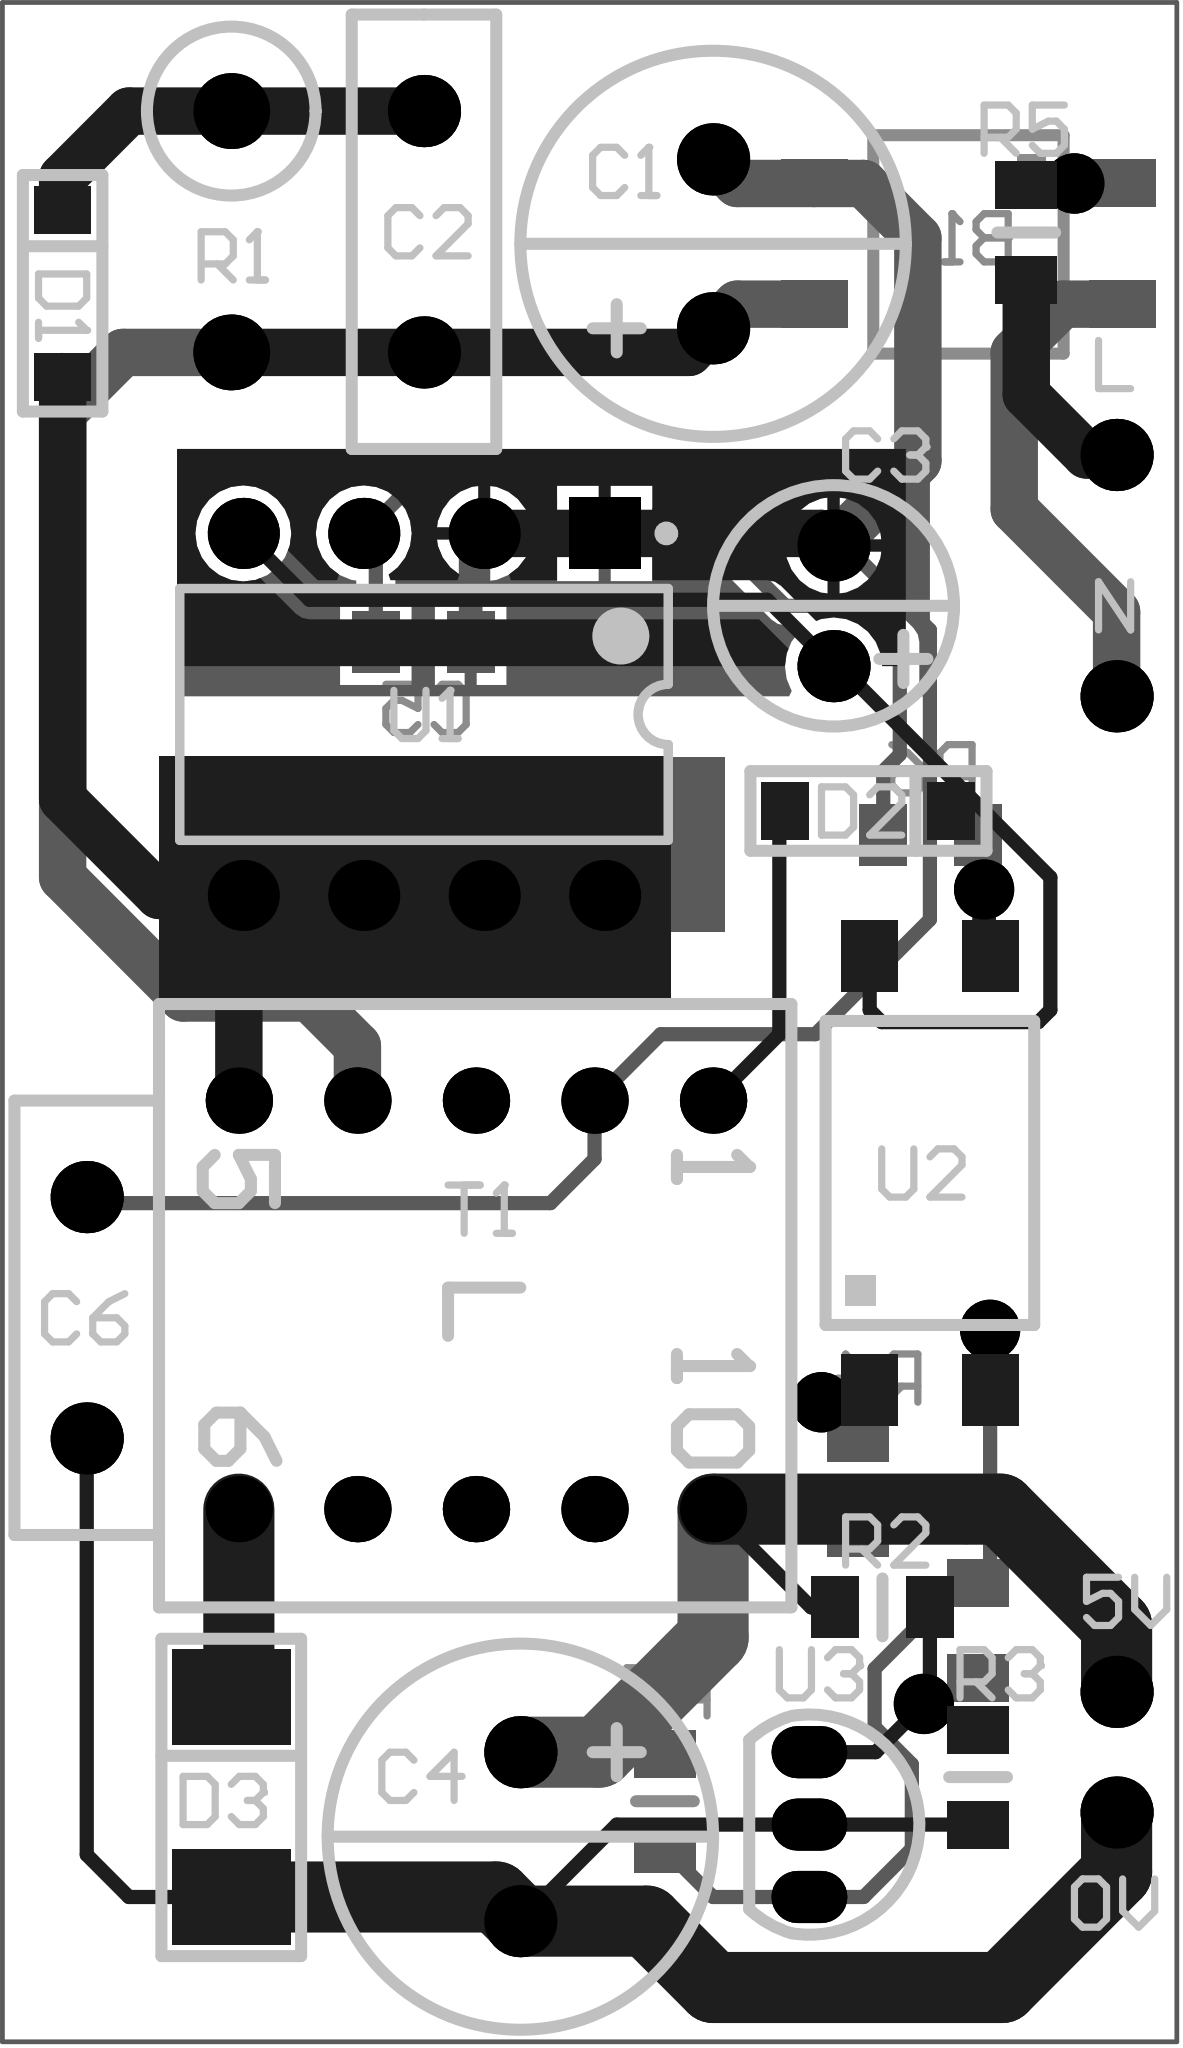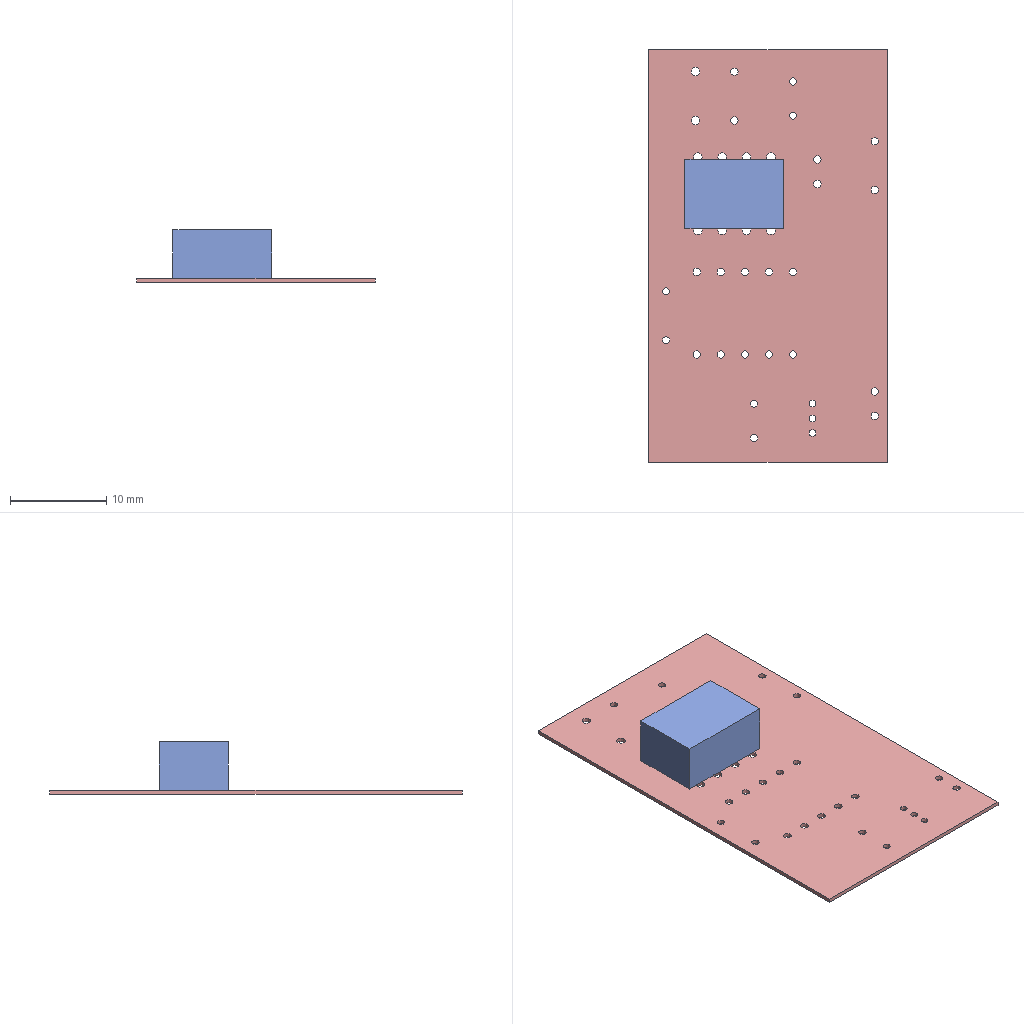Circuit board layout | Altium Designer | box 24.8 x 42.9 x 5.5 mm
Layer stack:
# Altium Designer layer stack of  (unit mm; dielectric type: 0 none, 1 core, 2 prepreg, 3 surface material)
index,name,kind,layer,copper_thickness_mm,dielectric_type,dielectric_thickness_mm,dielectric_material,dielectric_constant
0,Top Paste,other,,,,,,
1,Top Overlay,other,,,,,,
2,Top Solder,dielectric,,,3,0.0102,Solder Resist,3.5
3,Top Layer,copper,Top Layer,0.0356,,,,
4,Dielectric1,dielectric,,,0,0.32,FR-4,4.8
5,Bottom Layer,copper,Bottom Layer,0.0356,,,,
6,Bottom Solder,dielectric,,,3,0.0102,Solder Resist,3.5
7,Bottom Overlay,other,,,,,,
8,Bottom Paste,other,,,,,,
# drill layer pairs: low layer,high layer
drill_pair,Top Layer,Bottom Layer
Part placement:
Designator,Comment,Layer,Footprint,Center-X(mm),Center-Y(mm),Rotation
U1,AP8012,TopLayer,DIP-8,43.18,120.904,270
R7,1K,BottomLayer,0805_Res,48.26,98.028,90
U3,TL431,TopLayer,TO-92,51.308,97.536,270
U2,PC817,TopLayer,SOP4-PC817,53.848,111.252,90
T1,EE13,TopLayer,EE13_5+5_L,44.276,108.476,270
R6,8.2K,BottomLayer,0805_Res,53.864,118.364,360
R5,0R,TopLayer,0805_Res,55.88,131.048,90
R4,470R,BottomLayer,0805_Res,52.324,104.664,270
R3,1K,TopLayer,0805_Res,54.864,98.536,90
R2,1K,TopLayer,0805_Res,52.848,102.108,180
R1,33K/1W,TopLayer,1W_Res_L,39.116,131.064,270
D3,SS34,TopLayer,DO_214AC/SMA,39.116,98.112,90
D2,F7,TopLayer,SOD-123,52.55,118.872,360
D1,F7,TopLayer,SOD-123,35.56,129.766,90
C7,10nF,BottomLayer,0805_Cap,54.864,101.616,270
C6,1nF/1KV,TopLayer,CAP_5mm,36.068,108.204,90
C5,10nF,BottomLayer,0805_Cap,43.164,122.428,360
C4,1000uF/10V,TopLayer,cap-8*14mm,45.212,97.282,270
C3,10uF/25V,TopLayer,cap-5*12mm,51.816,123.19,90
C2,2.2nF/1KV,TopLayer,CAP_5mm,43.18,131.064,270
C1,4.7uF/400V,TopLayer,cap-8*14mm,49.276,130.81,90
B1,MB6S,BottomLayer,SOP4,54.662,130.81,180
Pad and via stacks:
# Altium Designer via and pad stacks of  (unit mm). Each distinct definition once, with the count of objects using it.
# via: kind,start_layer,end_layer,hole_mm,diameter_mm,mode(0 simple;1 top-mid-bottom;2 full stack),diameter_per_layer,count,example_net
# pad: kind,layer,hole_mm,hole_type(0 round;1 square;2 slot),plating,top_size,top_shape(1 round;2 rect;3 octagon;9 rounded rect),mid_size,bottom_size,mode,footprint,size_per_layer,count,example
pad,Top Layer,0,0,plated,1x1.2,2,1x1.2,1x1.2,0,SOD-123,,4,D1.2
pad,Top Layer,0,0,plated,1x1.3,2,1x1.3,1x1.3,0,0805_Res,,6,R5.1
pad,Top Layer,0,0,plated,1.5x1.2,2,1.5x1.2,1.5x1.2,0,SOP4-PC817,,4,U2.1
pad,Top Layer,0,0,plated,2x2.5,2,2x2.5,2x2.5,0,DO_214AC/SMA,,2,D3.2
pad,Multi-Layer,0.9,0,plated,1.5x1.5,2,1.5x1.5,1.5x1.5,0,DIP-8,,1,U1.1
pad,Multi-Layer,0.9,0,plated,1.5x1.5,1,1.5x1.5,1.5x1.5,0,DIP-8,,7,U1.2
pad,Multi-Layer,0.762,0,plated,1.524x1.524,1,1.524x1.524,1.524x1.524,0,CAP_5mm,,4,C6.2
pad,Multi-Layer,0.9,0,plated,1.6x1.6,1,1.6x1.6,1.6x1.6,0,1W_Res_L,,2,R1.2
pad,Multi-Layer,0.762,0,plated,1.524x1.524,1,1.524x1.524,1.524x1.524,0,cap-8*14mm,,4,C1.2
pad,Multi-Layer,0.7,0,plated,1.1x1.6,1,1.1x1.6,1.1x1.6,0,TO-92,,3,U3.1
pad,Multi-Layer,0.8,0,plated,1.4x1.4,1,1.4x1.4,1.4x1.4,0,EE13_5+5_L,,10,T1.1
pad,Multi-Layer,0.762,0,plated,1.524x1.524,1,1.524x1.524,1.524x1.524,0,cap-5*12mm,,2,C3.1
pad,Multi-Layer,0.762,0,plated,1.524x1.524,1,1.524x1.524,1.524x1.524,0,,,4,0
pad,Bottom Layer,0,0,plated,1x1.3,2,1x1.3,1x1.3,0,0805_Res,,6,R7.1
pad,Bottom Layer,0,0,plated,1x1.3,2,1x1.3,1x1.3,0,0805_Cap,,4,C7.2
pad,Bottom Layer,0,0,plated,1.4x1,2,1.4x1,1.4x1,0,SOP4,,4,B1.1
via,Top Layer,Bottom Layer,0.7112,1.27,0,,5,NetR6_2
Copper pours:
name,layer,net,type(0 solid;1 hatched;2 none)
Bottom Layer-No Net,Bottom Layer,HGND,0
Bottom Layer-No Net,Top Layer,HGND,0
Design rules, without the lines most boards share:
# Altium Designer design rules of  (exported by Altium Designer, unit mm)
# columns: name | kind | enabled | priority | scope1 | scope2 | descriptor | typed fields (field=value)
Clearance | 0 | enabled | 1 | All | All | Clearance Constraint (Gap=0.254mm) (All),(All) | gap=0.254
PlaneConnect | 6 | enabled | 1 | All | All | Power Plane Connect Rule(Relief Connect )(Expansion=0.508mm) (Conductor Width=0.254mm) (Air Gap=0.254mm) (Entries=4) (All) | relief_conductor_width=0.254 relief_entries=4 relief_expansion=0.508
PlaneClearance | 12 | enabled | 1 | All | All | Power Plane Clearance (Clearance =0.508mm) (All) | clearance=0.508
PolygonConnect | 20 | enabled | 1 | All | All | Polygon Connect Rule(Relief Connect )(Conductor Width=0.254mm) (Relief Angle=90 Angle) (Entries=4) (Air Gap Width=0.254mm) (All),(All) | connect_style(0=relief,1=direct,2=none)=0 relief_conductor_width=0.254 relief_entries=4
Width | 2 | enabled | 1 | All | All | Width Constraint (Min=0.3mm) (Max=1.5mm) (Preferred=1mm) (All) |
RoutingCorners | 10 | enabled | 1 | All | All | Routing Corners (Style=45-Degree) (Min Setback=2.54mm) (Max Setback=2.54mm) (All) |
RoutingVias | 11 | enabled | 1 | All | All | Routing Via (MinHoleWidth=0.711mm) (MaxHoleWidth=0.711mm) (PreferredHoleWidth=0.711mm) (MinWidth=1.27mm) (MaxWidth=1.27mm) (PreferedWidth=1.27mm) (All) | via_min_hole=0.7112 via_max_hole=0.7112 via_preferred_diameter=1.27 via_preferred_hole=0.7112
PasteMaskExpansion | 14 | enabled | 1 | All | All | Paste Mask Expansion (Expansion =0mm) (All) | expansion=0
SolderMaskExpansion | 13 | enabled | 1 | All | All | Solder Mask Expansion (Expansion =0.102mm) (All) | expansion=0.1016
ComponentClearance | 24 | enabled | 1 | All | All | Component Clearance Constraint ( Horizontal Gap = 0.254mm, Vertical Gap = 0.254mm ) (All),(All)  | gap=0.254
Height | 50 | enabled | 1 | All | All | Height Constraint (Min=0mm) (Max=25.4mm) (Prefered=12.7mm) (All) | min_height=0 max_height=25.4
HoleSize | 42 | enabled | 1 | All | All | Hole Size Constraint (Min=0.025mm) (Max=2.54mm) (All) |
DiffPairsRouting | 51 | enabled | 1 | All | All | Differential Pairs Uncoupled Length using the Gap Constraints (Min=0.254mm) (Max=0.254mm) (Prefered=0.254mm)  and Width Constraints (Min=0.381mm) (Max=0.381mm) (Prefered=0.381mm) (All) |
HoleToHoleClearance | 52 | enabled | 1 | All | All | Hole To Hole Clearance (Gap=0.254mm) (All),(All) | gap=0.254
MinimumSolderMaskSliver | 53 | enabled | 1 | All | All | Minimum Solder Mask Sliver (Gap=0.254mm) (All),(All) |
SilkscreenOverComponentPads | 54 | enabled | 1 | IsPad | All | Silk To Solder Mask (Clearance=0.254mm) (IsPad),(All) |
SilkToSilkClearance | 55 | enabled | 1 | All | All | Silk to Silk (Clearance=0.254mm) (All),(All) |
NetAntennae | 56 | enabled | 1 | All | All | Net Antennae (Tolerance=0mm) (All) |
Classes set for this board:
# Altium Designer classes of  (member kind: 0 net, 1 component, 2 from-to, 3 pad, 4 layer, 5 differential pair, 6 design channel, 7 polygon, 8 structure, 9 xSignal)
# columns: class name | member kind | superclass | members
5V1A_SMPS | 1 | no | B1; C1; C2; C3; C4; C5; C6; C7; D1; D2; D3; R1; R2; R3; R4; R5; R6; T1; U1; U2; U3; R7;